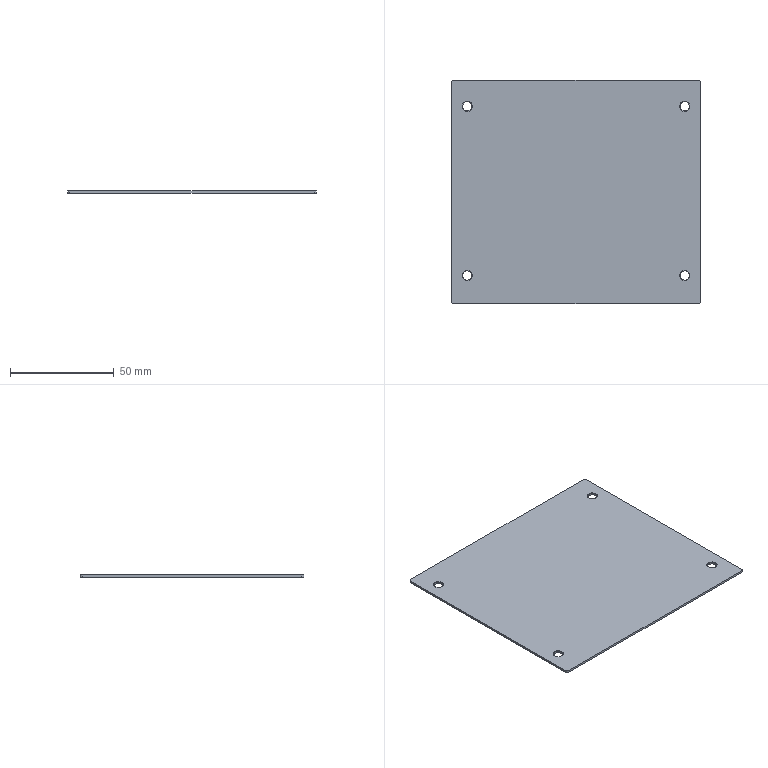Part | NX | 1 solid | 26 faces | box 120 x 108 x 1 mm | volume 12894 mm3 | cylinder 12 | cone 8 | plane 6 | commonest cylinder face diameters 4.5 x8 2 x4
STEP:
#1=CARTESIAN_POINT('',(1772.,9.5,60.5));
#2=VERTEX_POINT('',#1);
#3=CARTESIAN_POINT('',(1772.,9.5,61.5));
#4=VERTEX_POINT('',#3);
#5=CARTESIAN_POINT('',(1772.,9.5,61.5));
#6=DIRECTION('',(0.,0.,1.));
#7=VECTOR('',#6,1000.);
#8=LINE('',#5,#7);
#9=EDGE_CURVE('',#2,#4,#8,.T.);
#10=ORIENTED_EDGE('',*,*,#9,.T.);
#11=CARTESIAN_POINT('',(1772.,-96.5,61.5));
#12=VERTEX_POINT('',#11);
#13=CARTESIAN_POINT('',(1772.,-31.878,61.5));
#14=DIRECTION('',(0.,1.,0.));
#15=VECTOR('',#14,1000.);
#16=LINE('',#13,#15);
#17=EDGE_CURVE('',#12,#4,#16,.T.);
#18=ORIENTED_EDGE('',*,*,#17,.F.);
#19=CARTESIAN_POINT('',(1772.,-96.5,60.5));
#20=VERTEX_POINT('',#19);
#21=CARTESIAN_POINT('',(1772.,-96.5,61.5));
#22=DIRECTION('',(0.,0.,-1.));
#23=VECTOR('',#22,1000.);
#24=LINE('',#21,#23);
#25=EDGE_CURVE('',#12,#20,#24,.T.);
#26=ORIENTED_EDGE('',*,*,#25,.T.);
#27=CARTESIAN_POINT('',(1772.,-31.878,60.5));
#28=DIRECTION('',(0.,1.,0.));
#29=VECTOR('',#28,1000.);
#30=LINE('',#27,#29);
#31=EDGE_CURVE('',#20,#2,#30,.T.);
#32=ORIENTED_EDGE('',*,*,#31,.T.);
#33=EDGE_LOOP('',(#10,#18,#26,#32));
#34=FACE_BOUND('',#33,.T.);
#35=CARTESIAN_POINT('',(1772.,-97.5,61.5));
#36=DIRECTION('',(1.,0.,0.));
#37=DIRECTION('',(0.,1.,0.));
#38=AXIS2_PLACEMENT_3D('',#35,#36,#37);
#39=PLANE('',#38);
#40=ADVANCED_FACE('',(#34),#39,.T.);
#41=CARTESIAN_POINT('',(1653.,-97.5,61.5));
#42=VERTEX_POINT('',#41);
#43=CARTESIAN_POINT('',(1653.,-97.5,60.5));
#44=VERTEX_POINT('',#43);
#45=CARTESIAN_POINT('',(1653.,-97.5,61.5));
#46=DIRECTION('',(0.,0.,-1.));
#47=VECTOR('',#46,1000.);
#48=LINE('',#45,#47);
#49=EDGE_CURVE('',#42,#44,#48,.T.);
#50=ORIENTED_EDGE('',*,*,#49,.T.);
#51=CARTESIAN_POINT('',(1771.,-97.5,60.5));
#52=VERTEX_POINT('',#51);
#53=CARTESIAN_POINT('',(1652.,-97.5,60.5));
#54=DIRECTION('',(1.,0.,0.));
#55=VECTOR('',#54,1000.);
#56=LINE('',#53,#55);
#57=EDGE_CURVE('',#44,#52,#56,.T.);
#58=ORIENTED_EDGE('',*,*,#57,.T.);
#59=CARTESIAN_POINT('',(1771.,-97.5,61.5));
#60=VERTEX_POINT('',#59);
#61=CARTESIAN_POINT('',(1771.,-97.5,61.5));
#62=DIRECTION('',(0.,0.,-1.));
#63=VECTOR('',#62,1000.);
#64=LINE('',#61,#63);
#65=EDGE_CURVE('',#60,#52,#64,.T.);
#66=ORIENTED_EDGE('',*,*,#65,.F.);
#67=CARTESIAN_POINT('',(1652.,-97.5,61.5));
#68=DIRECTION('',(1.,0.,0.));
#69=VECTOR('',#68,1000.);
#70=LINE('',#67,#69);
#71=EDGE_CURVE('',#42,#60,#70,.T.);
#72=ORIENTED_EDGE('',*,*,#71,.F.);
#73=EDGE_LOOP('',(#50,#58,#66,#72));
#74=FACE_BOUND('',#73,.T.);
#75=CARTESIAN_POINT('',(1652.,-97.5,61.5));
#76=DIRECTION('',(0.,-1.,0.));
#77=DIRECTION('',(0.,0.,-1.));
#78=AXIS2_PLACEMENT_3D('',#75,#76,#77);
#79=PLANE('',#78);
#80=ADVANCED_FACE('',(#74),#79,.T.);
#81=CARTESIAN_POINT('',(1652.,9.5,61.5));
#82=VERTEX_POINT('',#81);
#83=CARTESIAN_POINT('',(1652.,9.5,60.5));
#84=VERTEX_POINT('',#83);
#85=CARTESIAN_POINT('',(1652.,9.5,61.5));
#86=DIRECTION('',(0.,0.,-1.));
#87=VECTOR('',#86,1000.);
#88=LINE('',#85,#87);
#89=EDGE_CURVE('',#82,#84,#88,.T.);
#90=ORIENTED_EDGE('',*,*,#89,.T.);
#91=CARTESIAN_POINT('',(1652.,-96.5,60.5));
#92=VERTEX_POINT('',#91);
#93=CARTESIAN_POINT('',(1652.,-31.878,60.5));
#94=DIRECTION('',(0.,-1.,0.));
#95=VECTOR('',#94,1000.);
#96=LINE('',#93,#95);
#97=EDGE_CURVE('',#84,#92,#96,.T.);
#98=ORIENTED_EDGE('',*,*,#97,.T.);
#99=CARTESIAN_POINT('',(1652.,-96.5,61.5));
#100=VERTEX_POINT('',#99);
#101=CARTESIAN_POINT('',(1652.,-96.5,61.5));
#102=DIRECTION('',(0.,0.,-1.));
#103=VECTOR('',#102,1000.);
#104=LINE('',#101,#103);
#105=EDGE_CURVE('',#100,#92,#104,.T.);
#106=ORIENTED_EDGE('',*,*,#105,.F.);
#107=CARTESIAN_POINT('',(1652.,-31.878,61.5));
#108=DIRECTION('',(0.,-1.,0.));
#109=VECTOR('',#108,1000.);
#110=LINE('',#107,#109);
#111=EDGE_CURVE('',#82,#100,#110,.T.);
#112=ORIENTED_EDGE('',*,*,#111,.F.);
#113=EDGE_LOOP('',(#90,#98,#106,#112));
#114=FACE_BOUND('',#113,.T.);
#115=CARTESIAN_POINT('',(1652.,11.5,61.5));
#116=DIRECTION('',(-1.,0.,0.));
#117=DIRECTION('',(0.,0.,1.));
#118=AXIS2_PLACEMENT_3D('',#115,#116,#117);
#119=PLANE('',#118);
#120=ADVANCED_FACE('',(#114),#119,.T.);
#121=CARTESIAN_POINT('',(1771.,10.5,61.5));
#122=VERTEX_POINT('',#121);
#123=CARTESIAN_POINT('',(1653.,10.5,61.5));
#124=VERTEX_POINT('',#123);
#125=CARTESIAN_POINT('',(1765.12,10.5,61.5));
#126=DIRECTION('',(-1.,0.,0.));
#127=VECTOR('',#126,1000.);
#128=LINE('',#125,#127);
#129=EDGE_CURVE('',#122,#124,#128,.T.);
#130=ORIENTED_EDGE('',*,*,#129,.F.);
#131=CARTESIAN_POINT('',(1771.,10.5,60.5));
#132=VERTEX_POINT('',#131);
#133=CARTESIAN_POINT('',(1771.,10.5,61.5));
#134=DIRECTION('',(0.,0.,1.));
#135=VECTOR('',#134,1000.);
#136=LINE('',#133,#135);
#137=EDGE_CURVE('',#132,#122,#136,.T.);
#138=ORIENTED_EDGE('',*,*,#137,.F.);
#139=CARTESIAN_POINT('',(1653.,10.5,60.5));
#140=VERTEX_POINT('',#139);
#141=CARTESIAN_POINT('',(1765.12,10.5,60.5));
#142=DIRECTION('',(-1.,0.,0.));
#143=VECTOR('',#142,1000.);
#144=LINE('',#141,#143);
#145=EDGE_CURVE('',#132,#140,#144,.T.);
#146=ORIENTED_EDGE('',*,*,#145,.T.);
#147=CARTESIAN_POINT('',(1653.,10.5,61.5));
#148=DIRECTION('',(0.,0.,-1.));
#149=VECTOR('',#148,1000.);
#150=LINE('',#147,#149);
#151=EDGE_CURVE('',#124,#140,#150,.T.);
#152=ORIENTED_EDGE('',*,*,#151,.F.);
#153=EDGE_LOOP('',(#130,#138,#146,#152));
#154=FACE_BOUND('',#153,.T.);
#155=CARTESIAN_POINT('',(1772.,10.5,61.5));
#156=DIRECTION('',(0.,1.,0.));
#157=DIRECTION('',(1.,0.,0.));
#158=AXIS2_PLACEMENT_3D('',#155,#156,#157);
#159=PLANE('',#158);
#160=ADVANCED_FACE('',(#154),#159,.T.);
#161=CARTESIAN_POINT('',(1766.75,-2.125,61.3));
#162=VERTEX_POINT('',#161);
#163=CARTESIAN_POINT('',(1762.25,-2.125,61.3));
#164=VERTEX_POINT('',#163);
#165=CARTESIAN_POINT('',(1764.5,-2.125,61.3));
#166=DIRECTION('',(0.,0.,1.));
#167=DIRECTION('',(1.,0.,0.));
#168=AXIS2_PLACEMENT_3D('',#165,#166,#167);
#169=CIRCLE('',#168,2.25);
#170=EDGE_CURVE('',#162,#164,#169,.T.);
#171=ORIENTED_EDGE('',*,*,#170,.T.);
#172=CARTESIAN_POINT('',(1762.25,-2.125,60.5));
#173=VERTEX_POINT('',#172);
#174=CARTESIAN_POINT('',(1762.25,-2.125,61.5));
#175=DIRECTION('',(0.,0.,1.));
#176=VECTOR('',#175,1000.);
#177=LINE('',#174,#176);
#178=EDGE_CURVE('',#173,#164,#177,.T.);
#179=ORIENTED_EDGE('',*,*,#178,.F.);
#180=CARTESIAN_POINT('',(1766.75,-2.125,60.5));
#181=VERTEX_POINT('',#180);
#182=CARTESIAN_POINT('',(1764.5,-2.125,60.5));
#183=DIRECTION('',(0.,0.,1.));
#184=DIRECTION('',(1.,0.,0.));
#185=AXIS2_PLACEMENT_3D('',#182,#183,#184);
#186=CIRCLE('',#185,2.25);
#187=EDGE_CURVE('',#181,#173,#186,.T.);
#188=ORIENTED_EDGE('',*,*,#187,.F.);
#189=CARTESIAN_POINT('',(1766.75,-2.125,61.5));
#190=DIRECTION('',(0.,0.,1.));
#191=VECTOR('',#190,1000.);
#192=LINE('',#189,#191);
#193=EDGE_CURVE('',#181,#162,#192,.T.);
#194=ORIENTED_EDGE('',*,*,#193,.T.);
#195=EDGE_LOOP('',(#171,#179,#188,#194));
#196=FACE_BOUND('',#195,.T.);
#197=CARTESIAN_POINT('',(1764.5,-2.125,61.5));
#198=DIRECTION('',(0.,0.,1.));
#199=DIRECTION('',(1.,0.,0.));
#200=AXIS2_PLACEMENT_3D('',#197,#198,#199);
#201=CYLINDRICAL_SURFACE('',#200,2.25);
#202=ADVANCED_FACE('',(#196),#201,.F.);
#203=ORIENTED_EDGE('',*,*,#170,.F.);
#204=CARTESIAN_POINT('',(1766.95,-2.125,61.5));
#205=VERTEX_POINT('',#204);
#206=CARTESIAN_POINT('',(1766.75,-2.125,61.3));
#207=DIRECTION('',(0.7071,0.,0.7071));
#208=VECTOR('',#207,1000.);
#209=LINE('',#206,#208);
#210=EDGE_CURVE('',#162,#205,#209,.T.);
#211=ORIENTED_EDGE('',*,*,#210,.T.);
#212=CARTESIAN_POINT('',(1762.05,-2.125,61.5));
#213=VERTEX_POINT('',#212);
#214=CARTESIAN_POINT('',(1764.5,-2.125,61.5));
#215=DIRECTION('',(0.,0.,1.));
#216=DIRECTION('',(1.,0.,0.));
#217=AXIS2_PLACEMENT_3D('',#214,#215,#216);
#218=CIRCLE('',#217,2.45);
#219=EDGE_CURVE('',#205,#213,#218,.T.);
#220=ORIENTED_EDGE('',*,*,#219,.T.);
#221=CARTESIAN_POINT('',(1762.25,-2.125,61.3));
#222=DIRECTION('',(-0.7071,0.,0.7071));
#223=VECTOR('',#222,1000.);
#224=LINE('',#221,#223);
#225=EDGE_CURVE('',#164,#213,#224,.T.);
#226=ORIENTED_EDGE('',*,*,#225,.F.);
#227=EDGE_LOOP('',(#203,#211,#220,#226));
#228=FACE_BOUND('',#227,.T.);
#229=CARTESIAN_POINT('',(1764.5,-2.125,61.3));
#230=DIRECTION('',(0.,0.,1.));
#231=DIRECTION('',(1.,0.,0.));
#232=AXIS2_PLACEMENT_3D('',#229,#230,#231);
#233=CONICAL_SURFACE('',#232,2.25,0.7854);
#234=ADVANCED_FACE('',(#228),#233,.F.);
#235=ORIENTED_EDGE('',*,*,#25,.F.);
#236=CARTESIAN_POINT('',(1771.,-96.5,61.5));
#237=DIRECTION('',(0.,0.,-1.));
#238=DIRECTION('',(-1.,0.,0.));
#239=AXIS2_PLACEMENT_3D('',#236,#237,#238);
#240=CIRCLE('',#239,1.);
#241=EDGE_CURVE('',#12,#60,#240,.T.);
#242=ORIENTED_EDGE('',*,*,#241,.T.);
#243=ORIENTED_EDGE('',*,*,#65,.T.);
#244=CARTESIAN_POINT('',(1771.,-96.5,60.5));
#245=DIRECTION('',(0.,0.,-1.));
#246=DIRECTION('',(-1.,0.,0.));
#247=AXIS2_PLACEMENT_3D('',#244,#245,#246);
#248=CIRCLE('',#247,1.);
#249=EDGE_CURVE('',#20,#52,#248,.T.);
#250=ORIENTED_EDGE('',*,*,#249,.F.);
#251=EDGE_LOOP('',(#235,#242,#243,#250));
#252=FACE_BOUND('',#251,.T.);
#253=CARTESIAN_POINT('',(1771.,-96.5,61.5));
#254=DIRECTION('',(0.,0.,-1.));
#255=DIRECTION('',(-1.,0.,0.));
#256=AXIS2_PLACEMENT_3D('',#253,#254,#255);
#257=CYLINDRICAL_SURFACE('',#256,1.);
#258=ADVANCED_FACE('',(#252),#257,.T.);
#259=ORIENTED_EDGE('',*,*,#49,.F.);
#260=CARTESIAN_POINT('',(1653.,-96.5,61.5));
#261=DIRECTION('',(0.,0.,-1.));
#262=DIRECTION('',(-1.,0.,0.));
#263=AXIS2_PLACEMENT_3D('',#260,#261,#262);
#264=CIRCLE('',#263,1.);
#265=EDGE_CURVE('',#42,#100,#264,.T.);
#266=ORIENTED_EDGE('',*,*,#265,.T.);
#267=ORIENTED_EDGE('',*,*,#105,.T.);
#268=CARTESIAN_POINT('',(1653.,-96.5,60.5));
#269=DIRECTION('',(0.,0.,-1.));
#270=DIRECTION('',(-1.,0.,0.));
#271=AXIS2_PLACEMENT_3D('',#268,#269,#270);
#272=CIRCLE('',#271,1.);
#273=EDGE_CURVE('',#44,#92,#272,.T.);
#274=ORIENTED_EDGE('',*,*,#273,.F.);
#275=EDGE_LOOP('',(#259,#266,#267,#274));
#276=FACE_BOUND('',#275,.T.);
#277=CARTESIAN_POINT('',(1653.,-96.5,61.5));
#278=DIRECTION('',(0.,0.,-1.));
#279=DIRECTION('',(-1.,0.,0.));
#280=AXIS2_PLACEMENT_3D('',#277,#278,#279);
#281=CYLINDRICAL_SURFACE('',#280,1.);
#282=ADVANCED_FACE('',(#276),#281,.T.);
#283=ORIENTED_EDGE('',*,*,#89,.F.);
#284=CARTESIAN_POINT('',(1653.,9.5,61.5));
#285=DIRECTION('',(0.,0.,-1.));
#286=DIRECTION('',(-1.,0.,0.));
#287=AXIS2_PLACEMENT_3D('',#284,#285,#286);
#288=CIRCLE('',#287,1.);
#289=EDGE_CURVE('',#82,#124,#288,.T.);
#290=ORIENTED_EDGE('',*,*,#289,.T.);
#291=ORIENTED_EDGE('',*,*,#151,.T.);
#292=CARTESIAN_POINT('',(1653.,9.5,60.5));
#293=DIRECTION('',(0.,0.,-1.));
#294=DIRECTION('',(-1.,0.,0.));
#295=AXIS2_PLACEMENT_3D('',#292,#293,#294);
#296=CIRCLE('',#295,1.);
#297=EDGE_CURVE('',#84,#140,#296,.T.);
#298=ORIENTED_EDGE('',*,*,#297,.F.);
#299=EDGE_LOOP('',(#283,#290,#291,#298));
#300=FACE_BOUND('',#299,.T.);
#301=CARTESIAN_POINT('',(1653.,9.5,61.5));
#302=DIRECTION('',(0.,0.,-1.));
#303=DIRECTION('',(-1.,0.,0.));
#304=AXIS2_PLACEMENT_3D('',#301,#302,#303);
#305=CYLINDRICAL_SURFACE('',#304,1.);
#306=ADVANCED_FACE('',(#300),#305,.T.);
#307=ORIENTED_EDGE('',*,*,#9,.F.);
#308=CARTESIAN_POINT('',(1771.,9.5,60.5));
#309=DIRECTION('',(0.,0.,1.));
#310=DIRECTION('',(1.,0.,0.));
#311=AXIS2_PLACEMENT_3D('',#308,#309,#310);
#312=CIRCLE('',#311,1.);
#313=EDGE_CURVE('',#2,#132,#312,.T.);
#314=ORIENTED_EDGE('',*,*,#313,.T.);
#315=ORIENTED_EDGE('',*,*,#137,.T.);
#316=CARTESIAN_POINT('',(1771.,9.5,61.5));
#317=DIRECTION('',(0.,0.,1.));
#318=DIRECTION('',(1.,0.,0.));
#319=AXIS2_PLACEMENT_3D('',#316,#317,#318);
#320=CIRCLE('',#319,1.);
#321=EDGE_CURVE('',#4,#122,#320,.T.);
#322=ORIENTED_EDGE('',*,*,#321,.F.);
#323=EDGE_LOOP('',(#307,#314,#315,#322));
#324=FACE_BOUND('',#323,.T.);
#325=CARTESIAN_POINT('',(1771.,9.5,61.5));
#326=DIRECTION('',(0.,0.,1.));
#327=DIRECTION('',(1.,0.,0.));
#328=AXIS2_PLACEMENT_3D('',#325,#326,#327);
#329=CYLINDRICAL_SURFACE('',#328,1.);
#330=ADVANCED_FACE('',(#324),#329,.T.);
#331=CARTESIAN_POINT('',(1657.25,-83.875,61.3));
#332=VERTEX_POINT('',#331);
#333=CARTESIAN_POINT('',(1661.75,-83.875,61.3));
#334=VERTEX_POINT('',#333);
#335=CARTESIAN_POINT('',(1659.5,-83.875,61.3));
#336=DIRECTION('',(0.,0.,1.));
#337=DIRECTION('',(1.,0.,0.));
#338=AXIS2_PLACEMENT_3D('',#335,#336,#337);
#339=CIRCLE('',#338,2.25);
#340=EDGE_CURVE('',#332,#334,#339,.T.);
#341=ORIENTED_EDGE('',*,*,#340,.F.);
#342=CARTESIAN_POINT('',(1657.05,-83.875,61.5));
#343=VERTEX_POINT('',#342);
#344=CARTESIAN_POINT('',(1657.25,-83.875,61.3));
#345=DIRECTION('',(-0.7071,0.,0.7071));
#346=VECTOR('',#345,1000.);
#347=LINE('',#344,#346);
#348=EDGE_CURVE('',#332,#343,#347,.T.);
#349=ORIENTED_EDGE('',*,*,#348,.T.);
#350=CARTESIAN_POINT('',(1661.95,-83.875,61.5));
#351=VERTEX_POINT('',#350);
#352=CARTESIAN_POINT('',(1659.5,-83.875,61.5));
#353=DIRECTION('',(0.,0.,1.));
#354=DIRECTION('',(1.,0.,0.));
#355=AXIS2_PLACEMENT_3D('',#352,#353,#354);
#356=CIRCLE('',#355,2.45);
#357=EDGE_CURVE('',#343,#351,#356,.T.);
#358=ORIENTED_EDGE('',*,*,#357,.T.);
#359=CARTESIAN_POINT('',(1661.75,-83.875,61.3));
#360=DIRECTION('',(0.7071,0.,0.7071));
#361=VECTOR('',#360,1000.);
#362=LINE('',#359,#361);
#363=EDGE_CURVE('',#334,#351,#362,.T.);
#364=ORIENTED_EDGE('',*,*,#363,.F.);
#365=EDGE_LOOP('',(#341,#349,#358,#364));
#366=FACE_BOUND('',#365,.T.);
#367=CARTESIAN_POINT('',(1659.5,-83.875,61.3));
#368=DIRECTION('',(0.,0.,1.));
#369=DIRECTION('',(1.,0.,0.));
#370=AXIS2_PLACEMENT_3D('',#367,#368,#369);
#371=CONICAL_SURFACE('',#370,2.25,0.7854);
#372=ADVANCED_FACE('',(#366),#371,.F.);
#373=ORIENTED_EDGE('',*,*,#111,.T.);
#374=ORIENTED_EDGE('',*,*,#265,.F.);
#375=ORIENTED_EDGE('',*,*,#71,.T.);
#376=ORIENTED_EDGE('',*,*,#241,.F.);
#377=ORIENTED_EDGE('',*,*,#17,.T.);
#378=ORIENTED_EDGE('',*,*,#321,.T.);
#379=ORIENTED_EDGE('',*,*,#129,.T.);
#380=ORIENTED_EDGE('',*,*,#289,.F.);
#381=EDGE_LOOP('',(#373,#374,#375,#376,#377,#378,#379,#380));
#382=FACE_BOUND('',#381,.T.);
#383=CARTESIAN_POINT('',(1764.5,-2.125,61.5));
#384=DIRECTION('',(0.,0.,1.));
#385=DIRECTION('',(1.,0.,0.));
#386=AXIS2_PLACEMENT_3D('',#383,#384,#385);
#387=CIRCLE('',#386,2.45);
#388=EDGE_CURVE('',#213,#205,#387,.T.);
#389=ORIENTED_EDGE('',*,*,#388,.F.);
#390=ORIENTED_EDGE('',*,*,#219,.F.);
#391=EDGE_LOOP('',(#389,#390));
#392=FACE_BOUND('',#391,.T.);
#393=ORIENTED_EDGE('',*,*,#357,.F.);
#394=CARTESIAN_POINT('',(1659.5,-83.875,61.5));
#395=DIRECTION('',(0.,0.,1.));
#396=DIRECTION('',(1.,0.,0.));
#397=AXIS2_PLACEMENT_3D('',#394,#395,#396);
#398=CIRCLE('',#397,2.45);
#399=EDGE_CURVE('',#351,#343,#398,.T.);
#400=ORIENTED_EDGE('',*,*,#399,.F.);
#401=EDGE_LOOP('',(#393,#400));
#402=FACE_BOUND('',#401,.T.);
#403=CARTESIAN_POINT('',(1766.95,-83.875,61.5));
#404=VERTEX_POINT('',#403);
#405=CARTESIAN_POINT('',(1762.05,-83.875,61.5));
#406=VERTEX_POINT('',#405);
#407=CARTESIAN_POINT('',(1764.5,-83.875,61.5));
#408=DIRECTION('',(0.,0.,1.));
#409=DIRECTION('',(1.,0.,0.));
#410=AXIS2_PLACEMENT_3D('',#407,#408,#409);
#411=CIRCLE('',#410,2.45);
#412=EDGE_CURVE('',#404,#406,#411,.T.);
#413=ORIENTED_EDGE('',*,*,#412,.F.);
#414=CARTESIAN_POINT('',(1764.5,-83.875,61.5));
#415=DIRECTION('',(0.,0.,1.));
#416=DIRECTION('',(1.,0.,0.));
#417=AXIS2_PLACEMENT_3D('',#414,#415,#416);
#418=CIRCLE('',#417,2.45);
#419=EDGE_CURVE('',#406,#404,#418,.T.);
#420=ORIENTED_EDGE('',*,*,#419,.F.);
#421=EDGE_LOOP('',(#413,#420));
#422=FACE_BOUND('',#421,.T.);
#423=CARTESIAN_POINT('',(1657.05,-2.125,61.5));
#424=VERTEX_POINT('',#423);
#425=CARTESIAN_POINT('',(1661.95,-2.125,61.5));
#426=VERTEX_POINT('',#425);
#427=CARTESIAN_POINT('',(1659.5,-2.125,61.5));
#428=DIRECTION('',(0.,0.,1.));
#429=DIRECTION('',(1.,0.,0.));
#430=AXIS2_PLACEMENT_3D('',#427,#428,#429);
#431=CIRCLE('',#430,2.45);
#432=EDGE_CURVE('',#424,#426,#431,.T.);
#433=ORIENTED_EDGE('',*,*,#432,.F.);
#434=CARTESIAN_POINT('',(1659.5,-2.125,61.5));
#435=DIRECTION('',(0.,0.,1.));
#436=DIRECTION('',(1.,0.,0.));
#437=AXIS2_PLACEMENT_3D('',#434,#435,#436);
#438=CIRCLE('',#437,2.45);
#439=EDGE_CURVE('',#426,#424,#438,.T.);
#440=ORIENTED_EDGE('',*,*,#439,.F.);
#441=EDGE_LOOP('',(#433,#440));
#442=FACE_BOUND('',#441,.T.);
#443=CARTESIAN_POINT('',(1765.12,-31.878,61.5));
#444=DIRECTION('',(0.,0.,1.));
#445=DIRECTION('',(1.,0.,0.));
#446=AXIS2_PLACEMENT_3D('',#443,#444,#445);
#447=PLANE('',#446);
#448=ADVANCED_FACE('',(#382,#392,#402,#422,#442),#447,.T.);
#449=ORIENTED_EDGE('',*,*,#145,.F.);
#450=ORIENTED_EDGE('',*,*,#313,.F.);
#451=ORIENTED_EDGE('',*,*,#31,.F.);
#452=ORIENTED_EDGE('',*,*,#249,.T.);
#453=ORIENTED_EDGE('',*,*,#57,.F.);
#454=ORIENTED_EDGE('',*,*,#273,.T.);
#455=ORIENTED_EDGE('',*,*,#97,.F.);
#456=ORIENTED_EDGE('',*,*,#297,.T.);
#457=EDGE_LOOP('',(#449,#450,#451,#452,#453,#454,#455,#456));
#458=FACE_BOUND('',#457,.T.);
#459=ORIENTED_EDGE('',*,*,#187,.T.);
#460=CARTESIAN_POINT('',(1764.5,-2.125,60.5));
#461=DIRECTION('',(0.,0.,1.));
#462=DIRECTION('',(1.,0.,0.));
#463=AXIS2_PLACEMENT_3D('',#460,#461,#462);
#464=CIRCLE('',#463,2.25);
#465=EDGE_CURVE('',#173,#181,#464,.T.);
#466=ORIENTED_EDGE('',*,*,#465,.T.);
#467=EDGE_LOOP('',(#459,#466));
#468=FACE_BOUND('',#467,.T.);
#469=CARTESIAN_POINT('',(1657.25,-2.125,60.5));
#470=VERTEX_POINT('',#469);
#471=CARTESIAN_POINT('',(1661.75,-2.125,60.5));
#472=VERTEX_POINT('',#471);
#473=CARTESIAN_POINT('',(1659.5,-2.125,60.5));
#474=DIRECTION('',(0.,0.,1.));
#475=DIRECTION('',(1.,0.,0.));
#476=AXIS2_PLACEMENT_3D('',#473,#474,#475);
#477=CIRCLE('',#476,2.25);
#478=EDGE_CURVE('',#470,#472,#477,.T.);
#479=ORIENTED_EDGE('',*,*,#478,.T.);
#480=CARTESIAN_POINT('',(1659.5,-2.125,60.5));
#481=DIRECTION('',(0.,0.,1.));
#482=DIRECTION('',(1.,0.,0.));
#483=AXIS2_PLACEMENT_3D('',#480,#481,#482);
#484=CIRCLE('',#483,2.25);
#485=EDGE_CURVE('',#472,#470,#484,.T.);
#486=ORIENTED_EDGE('',*,*,#485,.T.);
#487=EDGE_LOOP('',(#479,#486));
#488=FACE_BOUND('',#487,.T.);
#489=CARTESIAN_POINT('',(1657.25,-83.875,60.5));
#490=VERTEX_POINT('',#489);
#491=CARTESIAN_POINT('',(1661.75,-83.875,60.5));
#492=VERTEX_POINT('',#491);
#493=CARTESIAN_POINT('',(1659.5,-83.875,60.5));
#494=DIRECTION('',(0.,0.,1.));
#495=DIRECTION('',(1.,0.,0.));
#496=AXIS2_PLACEMENT_3D('',#493,#494,#495);
#497=CIRCLE('',#496,2.25);
#498=EDGE_CURVE('',#490,#492,#497,.T.);
#499=ORIENTED_EDGE('',*,*,#498,.T.);
#500=CARTESIAN_POINT('',(1659.5,-83.875,60.5));
#501=DIRECTION('',(0.,0.,1.));
#502=DIRECTION('',(1.,0.,0.));
#503=AXIS2_PLACEMENT_3D('',#500,#501,#502);
#504=CIRCLE('',#503,2.25);
#505=EDGE_CURVE('',#492,#490,#504,.T.);
#506=ORIENTED_EDGE('',*,*,#505,.T.);
#507=EDGE_LOOP('',(#499,#506));
#508=FACE_BOUND('',#507,.T.);
#509=CARTESIAN_POINT('',(1762.25,-83.875,60.5));
#510=VERTEX_POINT('',#509);
#511=CARTESIAN_POINT('',(1766.75,-83.875,60.5));
#512=VERTEX_POINT('',#511);
#513=CARTESIAN_POINT('',(1764.5,-83.875,60.5));
#514=DIRECTION('',(0.,0.,1.));
#515=DIRECTION('',(1.,0.,0.));
#516=AXIS2_PLACEMENT_3D('',#513,#514,#515);
#517=CIRCLE('',#516,2.25);
#518=EDGE_CURVE('',#510,#512,#517,.T.);
#519=ORIENTED_EDGE('',*,*,#518,.T.);
#520=CARTESIAN_POINT('',(1764.5,-83.875,60.5));
#521=DIRECTION('',(0.,0.,1.));
#522=DIRECTION('',(1.,0.,0.));
#523=AXIS2_PLACEMENT_3D('',#520,#521,#522);
#524=CIRCLE('',#523,2.25);
#525=EDGE_CURVE('',#512,#510,#524,.T.);
#526=ORIENTED_EDGE('',*,*,#525,.T.);
#527=EDGE_LOOP('',(#519,#526));
#528=FACE_BOUND('',#527,.T.);
#529=CARTESIAN_POINT('',(1765.12,-31.878,60.5));
#530=DIRECTION('',(0.,0.,1.));
#531=DIRECTION('',(1.,0.,0.));
#532=AXIS2_PLACEMENT_3D('',#529,#530,#531);
#533=PLANE('',#532);
#534=ADVANCED_FACE('',(#458,#468,#488,#508,#528),#533,.F.);
#535=CARTESIAN_POINT('',(1766.75,-83.875,61.3));
#536=VERTEX_POINT('',#535);
#537=CARTESIAN_POINT('',(1762.25,-83.875,61.3));
#538=VERTEX_POINT('',#537);
#539=CARTESIAN_POINT('',(1764.5,-83.875,61.3));
#540=DIRECTION('',(0.,0.,1.));
#541=DIRECTION('',(1.,0.,0.));
#542=AXIS2_PLACEMENT_3D('',#539,#540,#541);
#543=CIRCLE('',#542,2.25);
#544=EDGE_CURVE('',#536,#538,#543,.T.);
#545=ORIENTED_EDGE('',*,*,#544,.T.);
#546=CARTESIAN_POINT('',(1762.25,-83.875,61.5));
#547=DIRECTION('',(0.,0.,1.));
#548=VECTOR('',#547,1000.);
#549=LINE('',#546,#548);
#550=EDGE_CURVE('',#538,#510,#549,.F.);
#551=ORIENTED_EDGE('',*,*,#550,.T.);
#552=ORIENTED_EDGE('',*,*,#525,.F.);
#553=CARTESIAN_POINT('',(1766.75,-83.875,61.5));
#554=DIRECTION('',(0.,0.,1.));
#555=VECTOR('',#554,1000.);
#556=LINE('',#553,#555);
#557=EDGE_CURVE('',#536,#512,#556,.F.);
#558=ORIENTED_EDGE('',*,*,#557,.F.);
#559=EDGE_LOOP('',(#545,#551,#552,#558));
#560=FACE_BOUND('',#559,.T.);
#561=CARTESIAN_POINT('',(1764.5,-83.875,61.5));
#562=DIRECTION('',(0.,0.,1.));
#563=DIRECTION('',(1.,0.,0.));
#564=AXIS2_PLACEMENT_3D('',#561,#562,#563);
#565=CYLINDRICAL_SURFACE('',#564,2.25);
#566=ADVANCED_FACE('',(#560),#565,.F.);
#567=ORIENTED_EDGE('',*,*,#412,.T.);
#568=CARTESIAN_POINT('',(1762.25,-83.875,61.3));
#569=DIRECTION('',(-0.7071,0.,0.7071));
#570=VECTOR('',#569,1000.);
#571=LINE('',#568,#570);
#572=EDGE_CURVE('',#538,#406,#571,.T.);
#573=ORIENTED_EDGE('',*,*,#572,.F.);
#574=ORIENTED_EDGE('',*,*,#544,.F.);
#575=CARTESIAN_POINT('',(1766.75,-83.875,61.3));
#576=DIRECTION('',(0.7071,0.,0.7071));
#577=VECTOR('',#576,1000.);
#578=LINE('',#575,#577);
#579=EDGE_CURVE('',#536,#404,#578,.T.);
#580=ORIENTED_EDGE('',*,*,#579,.T.);
#581=EDGE_LOOP('',(#567,#573,#574,#580));
#582=FACE_BOUND('',#581,.T.);
#583=CARTESIAN_POINT('',(1764.5,-83.875,61.3));
#584=DIRECTION('',(0.,0.,1.));
#585=DIRECTION('',(1.,0.,0.));
#586=AXIS2_PLACEMENT_3D('',#583,#584,#585);
#587=CONICAL_SURFACE('',#586,2.25,0.7854);
#588=ADVANCED_FACE('',(#582),#587,.F.);
#589=ORIENTED_EDGE('',*,*,#478,.F.);
#590=CARTESIAN_POINT('',(1657.25,-2.125,61.3));
#591=VERTEX_POINT('',#590);
#592=CARTESIAN_POINT('',(1657.25,-2.125,61.5));
#593=DIRECTION('',(0.,0.,1.));
#594=VECTOR('',#593,1000.);
#595=LINE('',#592,#594);
#596=EDGE_CURVE('',#470,#591,#595,.T.);
#597=ORIENTED_EDGE('',*,*,#596,.T.);
#598=CARTESIAN_POINT('',(1661.75,-2.125,61.3));
#599=VERTEX_POINT('',#598);
#600=CARTESIAN_POINT('',(1659.5,-2.125,61.3));
#601=DIRECTION('',(0.,0.,1.));
#602=DIRECTION('',(1.,0.,0.));
#603=AXIS2_PLACEMENT_3D('',#600,#601,#602);
#604=CIRCLE('',#603,2.25);
#605=EDGE_CURVE('',#591,#599,#604,.T.);
#606=ORIENTED_EDGE('',*,*,#605,.T.);
#607=CARTESIAN_POINT('',(1661.75,-2.125,61.5));
#608=DIRECTION('',(0.,0.,1.));
#609=VECTOR('',#608,1000.);
#610=LINE('',#607,#609);
#611=EDGE_CURVE('',#472,#599,#610,.T.);
#612=ORIENTED_EDGE('',*,*,#611,.F.);
#613=EDGE_LOOP('',(#589,#597,#606,#612));
#614=FACE_BOUND('',#613,.T.);
#615=CARTESIAN_POINT('',(1659.5,-2.125,61.5));
#616=DIRECTION('',(0.,0.,1.));
#617=DIRECTION('',(1.,0.,0.));
#618=AXIS2_PLACEMENT_3D('',#615,#616,#617);
#619=CYLINDRICAL_SURFACE('',#618,2.25);
#620=ADVANCED_FACE('',(#614),#619,.F.);
#621=ORIENTED_EDGE('',*,*,#605,.F.);
#622=CARTESIAN_POINT('',(1657.25,-2.125,61.3));
#623=DIRECTION('',(-0.7071,0.,0.7071));
#624=VECTOR('',#623,1000.);
#625=LINE('',#622,#624);
#626=EDGE_CURVE('',#591,#424,#625,.T.);
#627=ORIENTED_EDGE('',*,*,#626,.T.);
#628=ORIENTED_EDGE('',*,*,#432,.T.);
#629=CARTESIAN_POINT('',(1661.75,-2.125,61.3));
#630=DIRECTION('',(0.7071,0.,0.7071));
#631=VECTOR('',#630,1000.);
#632=LINE('',#629,#631);
#633=EDGE_CURVE('',#599,#426,#632,.T.);
#634=ORIENTED_EDGE('',*,*,#633,.F.);
#635=EDGE_LOOP('',(#621,#627,#628,#634));
#636=FACE_BOUND('',#635,.T.);
#637=CARTESIAN_POINT('',(1659.5,-2.125,61.3));
#638=DIRECTION('',(0.,0.,1.));
#639=DIRECTION('',(1.,0.,0.));
#640=AXIS2_PLACEMENT_3D('',#637,#638,#639);
#641=CONICAL_SURFACE('',#640,2.25,0.7854);
#642=ADVANCED_FACE('',(#636),#641,.F.);
#643=ORIENTED_EDGE('',*,*,#498,.F.);
#644=CARTESIAN_POINT('',(1657.25,-83.875,61.5));
#645=DIRECTION('',(0.,0.,1.));
#646=VECTOR('',#645,1000.);
#647=LINE('',#644,#646);
#648=EDGE_CURVE('',#490,#332,#647,.T.);
#649=ORIENTED_EDGE('',*,*,#648,.T.);
#650=ORIENTED_EDGE('',*,*,#340,.T.);
#651=CARTESIAN_POINT('',(1661.75,-83.875,61.5));
#652=DIRECTION('',(0.,0.,1.));
#653=VECTOR('',#652,1000.);
#654=LINE('',#651,#653);
#655=EDGE_CURVE('',#492,#334,#654,.T.);
#656=ORIENTED_EDGE('',*,*,#655,.F.);
#657=EDGE_LOOP('',(#643,#649,#650,#656));
#658=FACE_BOUND('',#657,.T.);
#659=CARTESIAN_POINT('',(1659.5,-83.875,61.5));
#660=DIRECTION('',(0.,0.,1.));
#661=DIRECTION('',(1.,0.,0.));
#662=AXIS2_PLACEMENT_3D('',#659,#660,#661);
#663=CYLINDRICAL_SURFACE('',#662,2.25);
#664=ADVANCED_FACE('',(#658),#663,.F.);
#665=ORIENTED_EDGE('',*,*,#579,.F.);
#666=CARTESIAN_POINT('',(1764.5,-83.875,61.3));
#667=DIRECTION('',(0.,0.,1.));
#668=DIRECTION('',(1.,0.,0.));
#669=AXIS2_PLACEMENT_3D('',#666,#667,#668);
#670=CIRCLE('',#669,2.25);
#671=EDGE_CURVE('',#538,#536,#670,.T.);
#672=ORIENTED_EDGE('',*,*,#671,.F.);
#673=ORIENTED_EDGE('',*,*,#572,.T.);
#674=ORIENTED_EDGE('',*,*,#419,.T.);
#675=EDGE_LOOP('',(#665,#672,#673,#674));
#676=FACE_BOUND('',#675,.T.);
#677=CARTESIAN_POINT('',(1764.5,-83.875,61.3));
#678=DIRECTION('',(0.,0.,1.));
#679=DIRECTION('',(1.,0.,0.));
#680=AXIS2_PLACEMENT_3D('',#677,#678,#679);
#681=CONICAL_SURFACE('',#680,2.25,0.7854);
#682=ADVANCED_FACE('',(#676),#681,.F.);
#683=ORIENTED_EDGE('',*,*,#193,.F.);
#684=ORIENTED_EDGE('',*,*,#465,.F.);
#685=ORIENTED_EDGE('',*,*,#178,.T.);
#686=CARTESIAN_POINT('',(1764.5,-2.125,61.3));
#687=DIRECTION('',(0.,0.,1.));
#688=DIRECTION('',(1.,0.,0.));
#689=AXIS2_PLACEMENT_3D('',#686,#687,#688);
#690=CIRCLE('',#689,2.25);
#691=EDGE_CURVE('',#164,#162,#690,.T.);
#692=ORIENTED_EDGE('',*,*,#691,.T.);
#693=EDGE_LOOP('',(#683,#684,#685,#692));
#694=FACE_BOUND('',#693,.T.);
#695=CARTESIAN_POINT('',(1764.5,-2.125,61.5));
#696=DIRECTION('',(0.,0.,1.));
#697=DIRECTION('',(1.,0.,0.));
#698=AXIS2_PLACEMENT_3D('',#695,#696,#697);
#699=CYLINDRICAL_SURFACE('',#698,2.25);
#700=ADVANCED_FACE('',(#694),#699,.F.);
#701=ORIENTED_EDGE('',*,*,#518,.F.);
#702=ORIENTED_EDGE('',*,*,#550,.F.);
#703=ORIENTED_EDGE('',*,*,#671,.T.);
#704=ORIENTED_EDGE('',*,*,#557,.T.);
#705=EDGE_LOOP('',(#701,#702,#703,#704));
#706=FACE_BOUND('',#705,.T.);
#707=CARTESIAN_POINT('',(1764.5,-83.875,61.5));
#708=DIRECTION('',(0.,0.,1.));
#709=DIRECTION('',(1.,0.,0.));
#710=AXIS2_PLACEMENT_3D('',#707,#708,#709);
#711=CYLINDRICAL_SURFACE('',#710,2.25);
#712=ADVANCED_FACE('',(#706),#711,.F.);
#713=ORIENTED_EDGE('',*,*,#388,.T.);
#714=ORIENTED_EDGE('',*,*,#210,.F.);
#715=ORIENTED_EDGE('',*,*,#691,.F.);
#716=ORIENTED_EDGE('',*,*,#225,.T.);
#717=EDGE_LOOP('',(#713,#714,#715,#716));
#718=FACE_BOUND('',#717,.T.);
#719=CARTESIAN_POINT('',(1764.5,-2.125,61.3));
#720=DIRECTION('',(0.,0.,1.));
#721=DIRECTION('',(1.,0.,0.));
#722=AXIS2_PLACEMENT_3D('',#719,#720,#721);
#723=CONICAL_SURFACE('',#722,2.25,0.7854);
#724=ADVANCED_FACE('',(#718),#723,.F.);
#725=ORIENTED_EDGE('',*,*,#363,.T.);
#726=ORIENTED_EDGE('',*,*,#399,.T.);
#727=ORIENTED_EDGE('',*,*,#348,.F.);
#728=CARTESIAN_POINT('',(1659.5,-83.875,61.3));
#729=DIRECTION('',(0.,0.,1.));
#730=DIRECTION('',(1.,0.,0.));
#731=AXIS2_PLACEMENT_3D('',#728,#729,#730);
#732=CIRCLE('',#731,2.25);
#733=EDGE_CURVE('',#334,#332,#732,.T.);
#734=ORIENTED_EDGE('',*,*,#733,.F.);
#735=EDGE_LOOP('',(#725,#726,#727,#734));
#736=FACE_BOUND('',#735,.T.);
#737=CARTESIAN_POINT('',(1659.5,-83.875,61.3));
#738=DIRECTION('',(0.,0.,1.));
#739=DIRECTION('',(1.,0.,0.));
#740=AXIS2_PLACEMENT_3D('',#737,#738,#739);
#741=CONICAL_SURFACE('',#740,2.25,0.7854);
#742=ADVANCED_FACE('',(#736),#741,.F.);
#743=ORIENTED_EDGE('',*,*,#655,.T.);
#744=ORIENTED_EDGE('',*,*,#733,.T.);
#745=ORIENTED_EDGE('',*,*,#648,.F.);
#746=ORIENTED_EDGE('',*,*,#505,.F.);
#747=EDGE_LOOP('',(#743,#744,#745,#746));
#748=FACE_BOUND('',#747,.T.);
#749=CARTESIAN_POINT('',(1659.5,-83.875,61.5));
#750=DIRECTION('',(0.,0.,1.));
#751=DIRECTION('',(1.,0.,0.));
#752=AXIS2_PLACEMENT_3D('',#749,#750,#751);
#753=CYLINDRICAL_SURFACE('',#752,2.25);
#754=ADVANCED_FACE('',(#748),#753,.F.);
#755=ORIENTED_EDGE('',*,*,#633,.T.);
#756=ORIENTED_EDGE('',*,*,#439,.T.);
#757=ORIENTED_EDGE('',*,*,#626,.F.);
#758=CARTESIAN_POINT('',(1659.5,-2.125,61.3));
#759=DIRECTION('',(0.,0.,1.));
#760=DIRECTION('',(1.,0.,0.));
#761=AXIS2_PLACEMENT_3D('',#758,#759,#760);
#762=CIRCLE('',#761,2.25);
#763=EDGE_CURVE('',#599,#591,#762,.T.);
#764=ORIENTED_EDGE('',*,*,#763,.F.);
#765=EDGE_LOOP('',(#755,#756,#757,#764));
#766=FACE_BOUND('',#765,.T.);
#767=CARTESIAN_POINT('',(1659.5,-2.125,61.3));
#768=DIRECTION('',(0.,0.,1.));
#769=DIRECTION('',(1.,0.,0.));
#770=AXIS2_PLACEMENT_3D('',#767,#768,#769);
#771=CONICAL_SURFACE('',#770,2.25,0.7854);
#772=ADVANCED_FACE('',(#766),#771,.F.);
#773=ORIENTED_EDGE('',*,*,#611,.T.);
#774=ORIENTED_EDGE('',*,*,#763,.T.);
#775=ORIENTED_EDGE('',*,*,#596,.F.);
#776=ORIENTED_EDGE('',*,*,#485,.F.);
#777=EDGE_LOOP('',(#773,#774,#775,#776));
#778=FACE_BOUND('',#777,.T.);
#779=CARTESIAN_POINT('',(1659.5,-2.125,61.5));
#780=DIRECTION('',(0.,0.,1.));
#781=DIRECTION('',(1.,0.,0.));
#782=AXIS2_PLACEMENT_3D('',#779,#780,#781);
#783=CYLINDRICAL_SURFACE('',#782,2.25);
#784=ADVANCED_FACE('',(#778),#783,.F.);
#785=CLOSED_SHELL('',(#40,#80,#120,#160,#202,#234,#258,#282,#306,#330,#372,#448,#534,#566,#588,#620,#642,#664,#682,#700,#712,#724,#742,#754,#772,#784));
#786=MANIFOLD_SOLID_BREP('',#785);
#787=(LENGTH_UNIT()NAMED_UNIT(*)SI_UNIT(.MILLI.,.METRE.));
#788=UNCERTAINTY_MEASURE_WITH_UNIT(LENGTH_MEASURE(0.00001),#787,'','');
#789=(NAMED_UNIT(*)PLANE_ANGLE_UNIT()SI_UNIT($,.RADIAN.));
#790=(NAMED_UNIT(*)SI_UNIT($,.STERADIAN.)SOLID_ANGLE_UNIT());
#791=(GEOMETRIC_REPRESENTATION_CONTEXT(3)GLOBAL_UNCERTAINTY_ASSIGNED_CONTEXT((#788))GLOBAL_UNIT_ASSIGNED_CONTEXT((#787,#789,#790))REPRESENTATION_CONTEXT('',''));
#792=ADVANCED_BREP_SHAPE_REPRESENTATION('',(#786),#791);